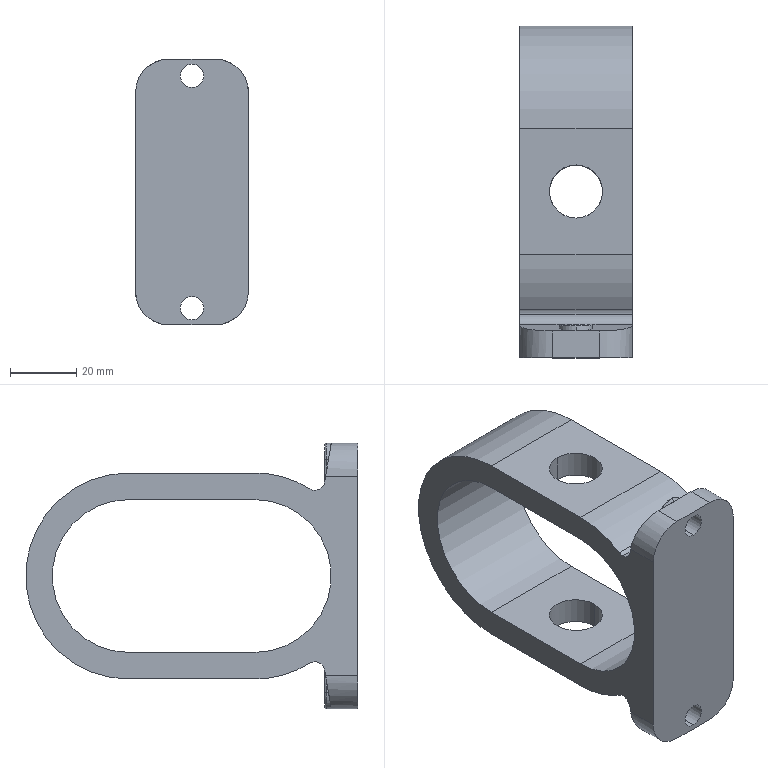Part | SolidWorks | features ICE 4, HoleWzd 3, Fillet 2, BaseBody 1 | 1 solid | 49 faces | box 34 x 100 x 80 mm | volume 78482 mm3 | cylinder 27 | plane 19 | torus 3 | commonest cylinder face diameters 1 x4 7 x4 16 x4 20 x4 6 x3 10 x3